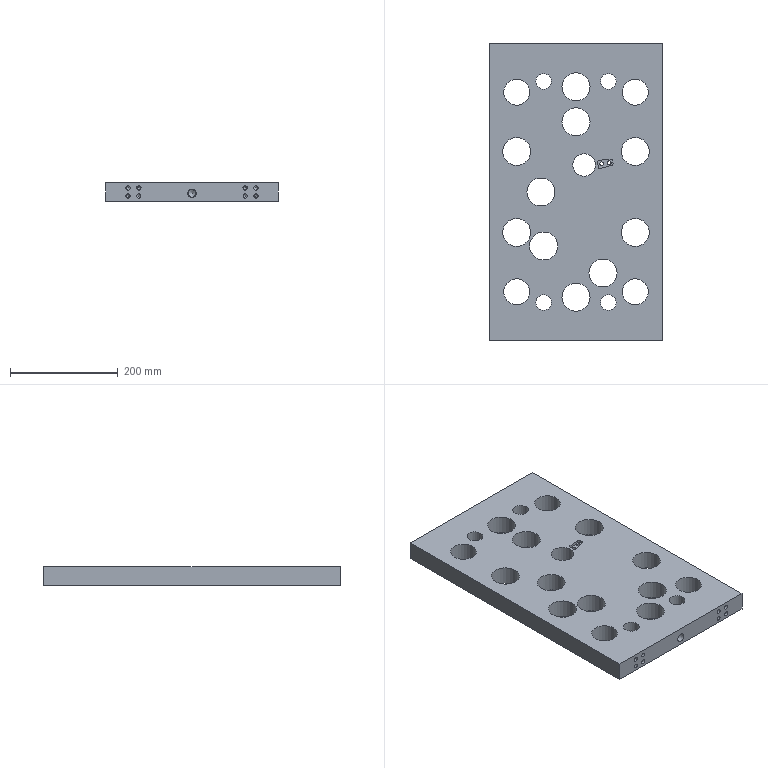Part | STEP file | 车灯-后视镜_id690_x_t | 1 solid | 132 faces | box 320 x 550 x 35 mm | volume 4960596 mm3 | cylinder 73 | plane 31 | cone 25 | other 2 | spline 1 | commonest cylinder face diameters 8 x16 52 x10 6.9 x8 3.2 x4 4 x4 6 x4